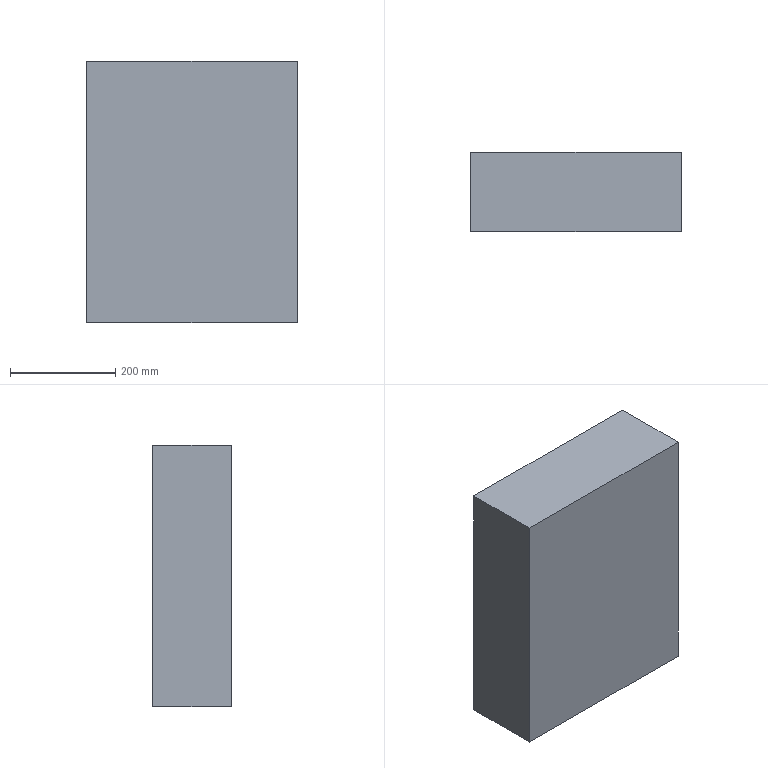Part | STEP file | Boss-Extrude 2-1 | 1 solid | 6 faces | box 400 x 150 x 498 mm | volume 29880000 mm3 | plane 6
STEP:
#1=CARTESIAN_POINT('',(-938.738,1949.264,3076.5));
#2=VERTEX_POINT('',#1);
#3=CARTESIAN_POINT('',(-938.738,1949.264,2578.5));
#4=VERTEX_POINT('',#3);
#5=CARTESIAN_POINT('',(-938.738,1949.264,2578.5));
#6=DIRECTION('',(0.,0.,-1.));
#7=VECTOR('',#6,1000.);
#8=LINE('',#5,#7);
#9=EDGE_CURVE('',#2,#4,#8,.T.);
#10=ORIENTED_EDGE('',*,*,#9,.T.);
#11=CARTESIAN_POINT('',(-1338.738,1949.264,2578.5));
#12=VERTEX_POINT('',#11);
#13=CARTESIAN_POINT('',(-1338.738,1949.264,2578.5));
#14=DIRECTION('',(1.,0.,0.));
#15=VECTOR('',#14,1000.);
#16=LINE('',#13,#15);
#17=EDGE_CURVE('',#12,#4,#16,.T.);
#18=ORIENTED_EDGE('',*,*,#17,.F.);
#19=CARTESIAN_POINT('',(-1338.738,1949.264,3076.5));
#20=VERTEX_POINT('',#19);
#21=CARTESIAN_POINT('',(-1338.738,1949.264,2578.5));
#22=DIRECTION('',(0.,0.,-1.));
#23=VECTOR('',#22,1000.);
#24=LINE('',#21,#23);
#25=EDGE_CURVE('',#20,#12,#24,.T.);
#26=ORIENTED_EDGE('',*,*,#25,.F.);
#27=CARTESIAN_POINT('',(-1338.738,1949.264,3076.5));
#28=DIRECTION('',(-1.,0.,0.));
#29=VECTOR('',#28,1000.);
#30=LINE('',#27,#29);
#31=EDGE_CURVE('',#2,#20,#30,.T.);
#32=ORIENTED_EDGE('',*,*,#31,.F.);
#33=EDGE_LOOP('',(#10,#18,#26,#32));
#34=FACE_OUTER_BOUND('',#33,.T.);
#35=CARTESIAN_POINT('',(-1338.738,1949.264,2578.5));
#36=DIRECTION('',(0.,-1.,0.));
#37=DIRECTION('',(-1.,0.,0.));
#38=AXIS2_PLACEMENT_3D('',#35,#36,#37);
#39=PLANE('',#38);
#40=ADVANCED_FACE('',(#34),#39,.F.);
#41=CARTESIAN_POINT('',(-938.738,1799.264,2578.5));
#42=VERTEX_POINT('',#41);
#43=CARTESIAN_POINT('',(-938.738,1949.264,2578.5));
#44=DIRECTION('',(0.,-1.,0.));
#45=VECTOR('',#44,1000.);
#46=LINE('',#43,#45);
#47=EDGE_CURVE('',#4,#42,#46,.T.);
#48=ORIENTED_EDGE('',*,*,#47,.T.);
#49=CARTESIAN_POINT('',(-1338.738,1799.264,2578.5));
#50=VERTEX_POINT('',#49);
#51=CARTESIAN_POINT('',(-1338.738,1799.264,2578.5));
#52=DIRECTION('',(1.,0.,0.));
#53=VECTOR('',#52,1000.);
#54=LINE('',#51,#53);
#55=EDGE_CURVE('',#50,#42,#54,.T.);
#56=ORIENTED_EDGE('',*,*,#55,.F.);
#57=CARTESIAN_POINT('',(-1338.738,1949.264,2578.5));
#58=DIRECTION('',(0.,-1.,0.));
#59=VECTOR('',#58,1000.);
#60=LINE('',#57,#59);
#61=EDGE_CURVE('',#12,#50,#60,.T.);
#62=ORIENTED_EDGE('',*,*,#61,.F.);
#63=ORIENTED_EDGE('',*,*,#17,.T.);
#64=EDGE_LOOP('',(#48,#56,#62,#63));
#65=FACE_OUTER_BOUND('',#64,.T.);
#66=CARTESIAN_POINT('',(-1338.738,1949.264,2578.5));
#67=DIRECTION('',(0.,0.,1.));
#68=DIRECTION('',(0.,-1.,0.));
#69=AXIS2_PLACEMENT_3D('',#66,#67,#68);
#70=PLANE('',#69);
#71=ADVANCED_FACE('',(#65),#70,.F.);
#72=CARTESIAN_POINT('',(-938.738,1799.264,3076.5));
#73=VERTEX_POINT('',#72);
#74=CARTESIAN_POINT('',(-938.738,1799.264,2578.5));
#75=DIRECTION('',(0.,0.,1.));
#76=VECTOR('',#75,1000.);
#77=LINE('',#74,#76);
#78=EDGE_CURVE('',#42,#73,#77,.T.);
#79=ORIENTED_EDGE('',*,*,#78,.T.);
#80=CARTESIAN_POINT('',(-1338.738,1799.264,3076.5));
#81=VERTEX_POINT('',#80);
#82=CARTESIAN_POINT('',(-938.738,1799.264,3076.5));
#83=DIRECTION('',(1.,0.,0.));
#84=VECTOR('',#83,1000.);
#85=LINE('',#82,#84);
#86=EDGE_CURVE('',#81,#73,#85,.T.);
#87=ORIENTED_EDGE('',*,*,#86,.F.);
#88=CARTESIAN_POINT('',(-1338.738,1799.264,2578.5));
#89=DIRECTION('',(0.,0.,1.));
#90=VECTOR('',#89,1000.);
#91=LINE('',#88,#90);
#92=EDGE_CURVE('',#50,#81,#91,.T.);
#93=ORIENTED_EDGE('',*,*,#92,.F.);
#94=ORIENTED_EDGE('',*,*,#55,.T.);
#95=EDGE_LOOP('',(#79,#87,#93,#94));
#96=FACE_OUTER_BOUND('',#95,.T.);
#97=CARTESIAN_POINT('',(-1338.738,1799.264,2578.5));
#98=DIRECTION('',(0.,1.,0.));
#99=DIRECTION('',(1.,0.,0.));
#100=AXIS2_PLACEMENT_3D('',#97,#98,#99);
#101=PLANE('',#100);
#102=ADVANCED_FACE('',(#96),#101,.F.);
#103=ORIENTED_EDGE('',*,*,#92,.T.);
#104=CARTESIAN_POINT('',(-1338.738,1799.264,3076.5));
#105=DIRECTION('',(0.,-1.,0.));
#106=VECTOR('',#105,1000.);
#107=LINE('',#104,#106);
#108=EDGE_CURVE('',#20,#81,#107,.T.);
#109=ORIENTED_EDGE('',*,*,#108,.F.);
#110=ORIENTED_EDGE('',*,*,#25,.T.);
#111=ORIENTED_EDGE('',*,*,#61,.T.);
#112=EDGE_LOOP('',(#103,#109,#110,#111));
#113=FACE_OUTER_BOUND('',#112,.T.);
#114=CARTESIAN_POINT('',(-1338.738,1874.264,2808.5));
#115=DIRECTION('',(-1.,0.,0.));
#116=DIRECTION('',(0.,0.,-1.));
#117=AXIS2_PLACEMENT_3D('',#114,#115,#116);
#118=PLANE('',#117);
#119=ADVANCED_FACE('',(#113),#118,.T.);
#120=ORIENTED_EDGE('',*,*,#9,.F.);
#121=CARTESIAN_POINT('',(-938.738,1949.264,3076.5));
#122=DIRECTION('',(0.,1.,0.));
#123=VECTOR('',#122,1000.);
#124=LINE('',#121,#123);
#125=EDGE_CURVE('',#73,#2,#124,.T.);
#126=ORIENTED_EDGE('',*,*,#125,.F.);
#127=ORIENTED_EDGE('',*,*,#78,.F.);
#128=ORIENTED_EDGE('',*,*,#47,.F.);
#129=EDGE_LOOP('',(#120,#126,#127,#128));
#130=FACE_OUTER_BOUND('',#129,.T.);
#131=CARTESIAN_POINT('',(-938.738,1874.264,2808.5));
#132=DIRECTION('',(-1.,0.,0.));
#133=DIRECTION('',(0.,0.,-1.));
#134=AXIS2_PLACEMENT_3D('',#131,#132,#133);
#135=PLANE('',#134);
#136=ADVANCED_FACE('',(#130),#135,.F.);
#137=ORIENTED_EDGE('',*,*,#108,.T.);
#138=ORIENTED_EDGE('',*,*,#86,.T.);
#139=ORIENTED_EDGE('',*,*,#125,.T.);
#140=ORIENTED_EDGE('',*,*,#31,.T.);
#141=EDGE_LOOP('',(#137,#138,#139,#140));
#142=FACE_OUTER_BOUND('',#141,.T.);
#143=CARTESIAN_POINT('',(-938.738,1874.264,3076.5));
#144=DIRECTION('',(0.,0.,-1.));
#145=DIRECTION('',(1.,0.,0.));
#146=AXIS2_PLACEMENT_3D('',#143,#144,#145);
#147=PLANE('',#146);
#148=ADVANCED_FACE('',(#142),#147,.F.);
#149=CLOSED_SHELL('',(#40,#71,#102,#119,#136,#148));
#150=MANIFOLD_SOLID_BREP('',#149);
#151=CARTESIAN_POINT('',(0.,0.,0.));
#152=DIRECTION('',(0.,0.,1.));
#153=DIRECTION('',(1.,0.,0.));
#154=AXIS2_PLACEMENT_3D('',#151,#152,#153);
#155=(LENGTH_UNIT()NAMED_UNIT(*)SI_UNIT(.MILLI.,.METRE.));
#156=UNCERTAINTY_MEASURE_WITH_UNIT(LENGTH_MEASURE(0.00001),#155,'','');
#157=(NAMED_UNIT(*)PLANE_ANGLE_UNIT()SI_UNIT($,.RADIAN.));
#158=(NAMED_UNIT(*)SI_UNIT($,.STERADIAN.)SOLID_ANGLE_UNIT());
#159=(GEOMETRIC_REPRESENTATION_CONTEXT(3)GLOBAL_UNCERTAINTY_ASSIGNED_CONTEXT((#156))GLOBAL_UNIT_ASSIGNED_CONTEXT((#155,#157,#158))REPRESENTATION_CONTEXT('',''));
#160=ADVANCED_BREP_SHAPE_REPRESENTATION('',(#150,#154),#159);